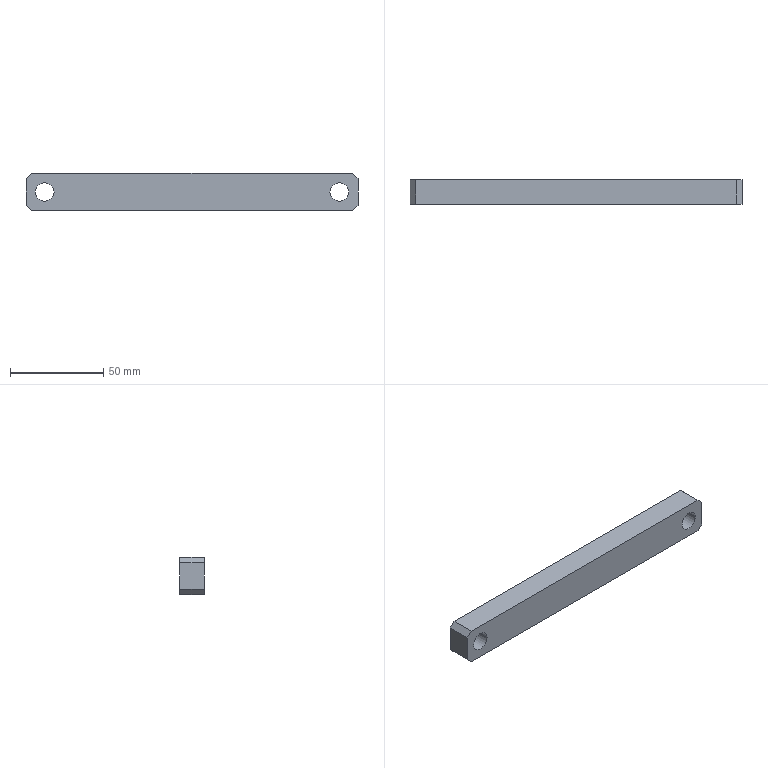Part | SolidWorks | features Chamfer 1, Extrusion 1, ICE 1, LPattern 1 | 1 solid | 14 faces | box 177.8 x 13 x 20 mm | volume 43952 mm3 | plane 10 | cylinder 4 | commonest cylinder face diameters 10 x4
STEP:
#1=CARTESIAN_POINT('',(83.9,-6.5,10.));
#2=VERTEX_POINT('',#1);
#3=CARTESIAN_POINT('',(73.9,-6.5,10.));
#4=VERTEX_POINT('',#3);
#5=CARTESIAN_POINT('',(78.9,-6.5,10.));
#6=DIRECTION('',(0.,1.,0.));
#7=DIRECTION('',(-1.,0.,0.));
#8=AXIS2_PLACEMENT_3D('',#5,#6,#7);
#9=CIRCLE('',#8,5.);
#10=EDGE_CURVE('',#2,#4,#9,.T.);
#11=ORIENTED_EDGE('',*,*,#10,.F.);
#12=CARTESIAN_POINT('',(83.9,6.5,10.));
#13=VERTEX_POINT('',#12);
#14=CARTESIAN_POINT('',(83.9,-6.5,10.));
#15=DIRECTION('',(0.,1.,0.));
#16=VECTOR('',#15,1000.);
#17=LINE('',#14,#16);
#18=EDGE_CURVE('',#2,#13,#17,.T.);
#19=ORIENTED_EDGE('',*,*,#18,.T.);
#20=CARTESIAN_POINT('',(73.9,6.5,10.));
#21=VERTEX_POINT('',#20);
#22=CARTESIAN_POINT('',(78.9,6.5,10.));
#23=DIRECTION('',(0.,1.,0.));
#24=DIRECTION('',(-1.,0.,0.));
#25=AXIS2_PLACEMENT_3D('',#22,#23,#24);
#26=CIRCLE('',#25,5.);
#27=EDGE_CURVE('',#13,#21,#26,.T.);
#28=ORIENTED_EDGE('',*,*,#27,.T.);
#29=CARTESIAN_POINT('',(73.9,-6.5,10.));
#30=DIRECTION('',(0.,1.,0.));
#31=VECTOR('',#30,1000.);
#32=LINE('',#29,#31);
#33=EDGE_CURVE('',#4,#21,#32,.T.);
#34=ORIENTED_EDGE('',*,*,#33,.F.);
#35=EDGE_LOOP('',(#11,#19,#28,#34));
#36=FACE_OUTER_BOUND('',#35,.T.);
#37=CARTESIAN_POINT('',(78.9,-6.5,10.));
#38=DIRECTION('',(0.,1.,0.));
#39=DIRECTION('',(-1.,0.,0.));
#40=AXIS2_PLACEMENT_3D('',#37,#38,#39);
#41=CYLINDRICAL_SURFACE('',#40,5.);
#42=ADVANCED_FACE('',(#36),#41,.F.);
#43=CARTESIAN_POINT('',(-73.9,-6.5,10.));
#44=VERTEX_POINT('',#43);
#45=CARTESIAN_POINT('',(-83.9,-6.5,10.));
#46=VERTEX_POINT('',#45);
#47=CARTESIAN_POINT('',(-78.9,-6.5,10.));
#48=DIRECTION('',(0.,1.,0.));
#49=DIRECTION('',(-1.,0.,0.));
#50=AXIS2_PLACEMENT_3D('',#47,#48,#49);
#51=CIRCLE('',#50,5.);
#52=EDGE_CURVE('',#44,#46,#51,.T.);
#53=ORIENTED_EDGE('',*,*,#52,.F.);
#54=CARTESIAN_POINT('',(-73.9,6.5,10.));
#55=VERTEX_POINT('',#54);
#56=CARTESIAN_POINT('',(-73.9,-6.5,10.));
#57=DIRECTION('',(0.,1.,0.));
#58=VECTOR('',#57,1000.);
#59=LINE('',#56,#58);
#60=EDGE_CURVE('',#44,#55,#59,.T.);
#61=ORIENTED_EDGE('',*,*,#60,.T.);
#62=CARTESIAN_POINT('',(-83.9,6.5,10.));
#63=VERTEX_POINT('',#62);
#64=CARTESIAN_POINT('',(-78.9,6.5,10.));
#65=DIRECTION('',(0.,1.,0.));
#66=DIRECTION('',(-1.,0.,0.));
#67=AXIS2_PLACEMENT_3D('',#64,#65,#66);
#68=CIRCLE('',#67,5.);
#69=EDGE_CURVE('',#55,#63,#68,.T.);
#70=ORIENTED_EDGE('',*,*,#69,.T.);
#71=CARTESIAN_POINT('',(-83.9,-6.5,10.));
#72=DIRECTION('',(0.,1.,0.));
#73=VECTOR('',#72,1000.);
#74=LINE('',#71,#73);
#75=EDGE_CURVE('',#46,#63,#74,.T.);
#76=ORIENTED_EDGE('',*,*,#75,.F.);
#77=EDGE_LOOP('',(#53,#61,#70,#76));
#78=FACE_OUTER_BOUND('',#77,.T.);
#79=CARTESIAN_POINT('',(-78.9,-6.5,10.));
#80=DIRECTION('',(0.,1.,0.));
#81=DIRECTION('',(-1.,0.,0.));
#82=AXIS2_PLACEMENT_3D('',#79,#80,#81);
#83=CYLINDRICAL_SURFACE('',#82,5.);
#84=ADVANCED_FACE('',(#78),#83,.F.);
#85=CARTESIAN_POINT('',(88.9,-6.5,17.));
#86=VERTEX_POINT('',#85);
#87=CARTESIAN_POINT('',(88.9,-6.5,3.));
#88=VERTEX_POINT('',#87);
#89=CARTESIAN_POINT('',(88.9,-6.5,20.));
#90=DIRECTION('',(0.,0.,-1.));
#91=VECTOR('',#90,1000.);
#92=LINE('',#89,#91);
#93=EDGE_CURVE('',#86,#88,#92,.T.);
#94=ORIENTED_EDGE('',*,*,#93,.T.);
#95=CARTESIAN_POINT('',(88.9,6.5,3.));
#96=VERTEX_POINT('',#95);
#97=CARTESIAN_POINT('',(88.9,6.5,3.));
#98=DIRECTION('',(0.,1.,0.));
#99=VECTOR('',#98,1000.);
#100=LINE('',#97,#99);
#101=EDGE_CURVE('',#88,#96,#100,.T.);
#102=ORIENTED_EDGE('',*,*,#101,.T.);
#103=CARTESIAN_POINT('',(88.9,6.5,17.));
#104=VERTEX_POINT('',#103);
#105=CARTESIAN_POINT('',(88.9,6.5,20.));
#106=DIRECTION('',(0.,0.,-1.));
#107=VECTOR('',#106,1000.);
#108=LINE('',#105,#107);
#109=EDGE_CURVE('',#104,#96,#108,.T.);
#110=ORIENTED_EDGE('',*,*,#109,.F.);
#111=CARTESIAN_POINT('',(88.9,-6.5,17.));
#112=DIRECTION('',(0.,-1.,0.));
#113=VECTOR('',#112,1000.);
#114=LINE('',#111,#113);
#115=EDGE_CURVE('',#104,#86,#114,.T.);
#116=ORIENTED_EDGE('',*,*,#115,.T.);
#117=EDGE_LOOP('',(#94,#102,#110,#116));
#118=FACE_OUTER_BOUND('',#117,.T.);
#119=CARTESIAN_POINT('',(88.9,6.5,20.));
#120=DIRECTION('',(-1.,0.,0.));
#121=DIRECTION('',(0.,0.,1.));
#122=AXIS2_PLACEMENT_3D('',#119,#120,#121);
#123=PLANE('',#122);
#124=ADVANCED_FACE('',(#118),#123,.F.);
#125=CARTESIAN_POINT('',(78.9,6.5,10.));
#126=DIRECTION('',(0.,1.,0.));
#127=DIRECTION('',(-1.,0.,0.));
#128=AXIS2_PLACEMENT_3D('',#125,#126,#127);
#129=CIRCLE('',#128,5.);
#130=EDGE_CURVE('',#21,#13,#129,.T.);
#131=ORIENTED_EDGE('',*,*,#130,.F.);
#132=ORIENTED_EDGE('',*,*,#27,.F.);
#133=EDGE_LOOP('',(#131,#132));
#134=FACE_BOUND('',#133,.T.);
#135=CARTESIAN_POINT('',(-78.9,6.5,10.));
#136=DIRECTION('',(0.,1.,0.));
#137=DIRECTION('',(-1.,0.,0.));
#138=AXIS2_PLACEMENT_3D('',#135,#136,#137);
#139=CIRCLE('',#138,5.);
#140=EDGE_CURVE('',#63,#55,#139,.T.);
#141=ORIENTED_EDGE('',*,*,#140,.F.);
#142=ORIENTED_EDGE('',*,*,#69,.F.);
#143=EDGE_LOOP('',(#141,#142));
#144=FACE_BOUND('',#143,.T.);
#145=ORIENTED_EDGE('',*,*,#109,.T.);
#146=CARTESIAN_POINT('',(85.9,6.5,0.));
#147=VERTEX_POINT('',#146);
#148=CARTESIAN_POINT('',(88.9,6.5,3.));
#149=DIRECTION('',(-0.7071,0.,-0.7071));
#150=VECTOR('',#149,1000.);
#151=LINE('',#148,#150);
#152=EDGE_CURVE('',#96,#147,#151,.T.);
#153=ORIENTED_EDGE('',*,*,#152,.T.);
#154=CARTESIAN_POINT('',(-85.9,6.5,0.));
#155=VERTEX_POINT('',#154);
#156=CARTESIAN_POINT('',(-88.9,6.5,0.));
#157=DIRECTION('',(-1.,0.,0.));
#158=VECTOR('',#157,1000.);
#159=LINE('',#156,#158);
#160=EDGE_CURVE('',#147,#155,#159,.T.);
#161=ORIENTED_EDGE('',*,*,#160,.T.);
#162=CARTESIAN_POINT('',(-88.9,6.5,3.));
#163=VERTEX_POINT('',#162);
#164=CARTESIAN_POINT('',(-88.9,6.5,3.));
#165=DIRECTION('',(-0.7071,0.,0.7071));
#166=VECTOR('',#165,1000.);
#167=LINE('',#164,#166);
#168=EDGE_CURVE('',#155,#163,#167,.T.);
#169=ORIENTED_EDGE('',*,*,#168,.T.);
#170=CARTESIAN_POINT('',(-88.9,6.5,17.));
#171=VERTEX_POINT('',#170);
#172=CARTESIAN_POINT('',(-88.9,6.5,20.));
#173=DIRECTION('',(0.,0.,-1.));
#174=VECTOR('',#173,1000.);
#175=LINE('',#172,#174);
#176=EDGE_CURVE('',#171,#163,#175,.T.);
#177=ORIENTED_EDGE('',*,*,#176,.F.);
#178=CARTESIAN_POINT('',(-85.9,6.5,20.));
#179=VERTEX_POINT('',#178);
#180=CARTESIAN_POINT('',(-85.9,6.5,20.));
#181=DIRECTION('',(0.7071,0.,0.7071));
#182=VECTOR('',#181,1000.);
#183=LINE('',#180,#182);
#184=EDGE_CURVE('',#171,#179,#183,.T.);
#185=ORIENTED_EDGE('',*,*,#184,.T.);
#186=CARTESIAN_POINT('',(85.9,6.5,20.));
#187=VERTEX_POINT('',#186);
#188=CARTESIAN_POINT('',(-88.9,6.5,20.));
#189=DIRECTION('',(-1.,0.,0.));
#190=VECTOR('',#189,1000.);
#191=LINE('',#188,#190);
#192=EDGE_CURVE('',#187,#179,#191,.T.);
#193=ORIENTED_EDGE('',*,*,#192,.F.);
#194=CARTESIAN_POINT('',(85.9,6.5,20.));
#195=DIRECTION('',(0.7071,0.,-0.7071));
#196=VECTOR('',#195,1000.);
#197=LINE('',#194,#196);
#198=EDGE_CURVE('',#187,#104,#197,.T.);
#199=ORIENTED_EDGE('',*,*,#198,.T.);
#200=EDGE_LOOP('',(#145,#153,#161,#169,#177,#185,#193,#199));
#201=FACE_OUTER_BOUND('',#200,.T.);
#202=CARTESIAN_POINT('',(-88.9,6.5,20.));
#203=DIRECTION('',(0.,-1.,0.));
#204=DIRECTION('',(0.,0.,-1.));
#205=AXIS2_PLACEMENT_3D('',#202,#203,#204);
#206=PLANE('',#205);
#207=ADVANCED_FACE('',(#134,#144,#201),#206,.F.);
#208=ORIENTED_EDGE('',*,*,#176,.T.);
#209=CARTESIAN_POINT('',(-88.9,-6.5,3.));
#210=VERTEX_POINT('',#209);
#211=CARTESIAN_POINT('',(-88.9,6.5,3.));
#212=DIRECTION('',(0.,-1.,0.));
#213=VECTOR('',#212,1000.);
#214=LINE('',#211,#213);
#215=EDGE_CURVE('',#163,#210,#214,.T.);
#216=ORIENTED_EDGE('',*,*,#215,.T.);
#217=CARTESIAN_POINT('',(-88.9,-6.5,17.));
#218=VERTEX_POINT('',#217);
#219=CARTESIAN_POINT('',(-88.9,-6.5,20.));
#220=DIRECTION('',(0.,0.,-1.));
#221=VECTOR('',#220,1000.);
#222=LINE('',#219,#221);
#223=EDGE_CURVE('',#218,#210,#222,.T.);
#224=ORIENTED_EDGE('',*,*,#223,.F.);
#225=CARTESIAN_POINT('',(-88.9,6.5,17.));
#226=DIRECTION('',(0.,1.,0.));
#227=VECTOR('',#226,1000.);
#228=LINE('',#225,#227);
#229=EDGE_CURVE('',#218,#171,#228,.T.);
#230=ORIENTED_EDGE('',*,*,#229,.T.);
#231=EDGE_LOOP('',(#208,#216,#224,#230));
#232=FACE_OUTER_BOUND('',#231,.T.);
#233=CARTESIAN_POINT('',(-88.9,6.5,20.));
#234=DIRECTION('',(1.,0.,0.));
#235=DIRECTION('',(0.,0.,-1.));
#236=AXIS2_PLACEMENT_3D('',#233,#234,#235);
#237=PLANE('',#236);
#238=ADVANCED_FACE('',(#232),#237,.F.);
#239=CARTESIAN_POINT('',(78.9,-6.5,10.));
#240=DIRECTION('',(0.,1.,0.));
#241=DIRECTION('',(-1.,0.,0.));
#242=AXIS2_PLACEMENT_3D('',#239,#240,#241);
#243=CIRCLE('',#242,5.);
#244=EDGE_CURVE('',#4,#2,#243,.T.);
#245=ORIENTED_EDGE('',*,*,#244,.T.);
#246=ORIENTED_EDGE('',*,*,#10,.T.);
#247=EDGE_LOOP('',(#245,#246));
#248=FACE_BOUND('',#247,.T.);
#249=CARTESIAN_POINT('',(-78.9,-6.5,10.));
#250=DIRECTION('',(0.,1.,0.));
#251=DIRECTION('',(-1.,0.,0.));
#252=AXIS2_PLACEMENT_3D('',#249,#250,#251);
#253=CIRCLE('',#252,5.);
#254=EDGE_CURVE('',#46,#44,#253,.T.);
#255=ORIENTED_EDGE('',*,*,#254,.T.);
#256=ORIENTED_EDGE('',*,*,#52,.T.);
#257=EDGE_LOOP('',(#255,#256));
#258=FACE_BOUND('',#257,.T.);
#259=CARTESIAN_POINT('',(-85.9,-6.5,0.));
#260=VERTEX_POINT('',#259);
#261=CARTESIAN_POINT('',(85.9,-6.5,0.));
#262=VERTEX_POINT('',#261);
#263=CARTESIAN_POINT('',(-88.9,-6.5,0.));
#264=DIRECTION('',(1.,0.,0.));
#265=VECTOR('',#264,1000.);
#266=LINE('',#263,#265);
#267=EDGE_CURVE('',#260,#262,#266,.T.);
#268=ORIENTED_EDGE('',*,*,#267,.T.);
#269=CARTESIAN_POINT('',(88.9,-6.5,3.));
#270=DIRECTION('',(0.7071,0.,0.7071));
#271=VECTOR('',#270,1000.);
#272=LINE('',#269,#271);
#273=EDGE_CURVE('',#262,#88,#272,.T.);
#274=ORIENTED_EDGE('',*,*,#273,.T.);
#275=ORIENTED_EDGE('',*,*,#93,.F.);
#276=CARTESIAN_POINT('',(85.9,-6.5,20.));
#277=VERTEX_POINT('',#276);
#278=CARTESIAN_POINT('',(85.9,-6.5,20.));
#279=DIRECTION('',(-0.7071,0.,0.7071));
#280=VECTOR('',#279,1000.);
#281=LINE('',#278,#280);
#282=EDGE_CURVE('',#86,#277,#281,.T.);
#283=ORIENTED_EDGE('',*,*,#282,.T.);
#284=CARTESIAN_POINT('',(-85.9,-6.5,20.));
#285=VERTEX_POINT('',#284);
#286=CARTESIAN_POINT('',(-88.9,-6.5,20.));
#287=DIRECTION('',(1.,0.,0.));
#288=VECTOR('',#287,1000.);
#289=LINE('',#286,#288);
#290=EDGE_CURVE('',#285,#277,#289,.T.);
#291=ORIENTED_EDGE('',*,*,#290,.F.);
#292=CARTESIAN_POINT('',(-85.9,-6.5,20.));
#293=DIRECTION('',(-0.7071,0.,-0.7071));
#294=VECTOR('',#293,1000.);
#295=LINE('',#292,#294);
#296=EDGE_CURVE('',#285,#218,#295,.T.);
#297=ORIENTED_EDGE('',*,*,#296,.T.);
#298=ORIENTED_EDGE('',*,*,#223,.T.);
#299=CARTESIAN_POINT('',(-88.9,-6.5,3.));
#300=DIRECTION('',(0.7071,0.,-0.7071));
#301=VECTOR('',#300,1000.);
#302=LINE('',#299,#301);
#303=EDGE_CURVE('',#210,#260,#302,.T.);
#304=ORIENTED_EDGE('',*,*,#303,.T.);
#305=EDGE_LOOP('',(#268,#274,#275,#283,#291,#297,#298,#304));
#306=FACE_OUTER_BOUND('',#305,.T.);
#307=CARTESIAN_POINT('',(-88.9,-6.5,20.));
#308=DIRECTION('',(0.,1.,0.));
#309=DIRECTION('',(0.,0.,1.));
#310=AXIS2_PLACEMENT_3D('',#307,#308,#309);
#311=PLANE('',#310);
#312=ADVANCED_FACE('',(#248,#258,#306),#311,.F.);
#313=ORIENTED_EDGE('',*,*,#192,.T.);
#314=CARTESIAN_POINT('',(-85.9,-6.5,20.));
#315=DIRECTION('',(0.,-1.,0.));
#316=VECTOR('',#315,1000.);
#317=LINE('',#314,#316);
#318=EDGE_CURVE('',#179,#285,#317,.T.);
#319=ORIENTED_EDGE('',*,*,#318,.T.);
#320=ORIENTED_EDGE('',*,*,#290,.T.);
#321=CARTESIAN_POINT('',(85.9,6.5,20.));
#322=DIRECTION('',(0.,1.,0.));
#323=VECTOR('',#322,1000.);
#324=LINE('',#321,#323);
#325=EDGE_CURVE('',#277,#187,#324,.T.);
#326=ORIENTED_EDGE('',*,*,#325,.T.);
#327=EDGE_LOOP('',(#313,#319,#320,#326));
#328=FACE_OUTER_BOUND('',#327,.T.);
#329=CARTESIAN_POINT('',(0.,0.,20.));
#330=DIRECTION('',(0.,0.,1.));
#331=DIRECTION('',(1.,0.,0.));
#332=AXIS2_PLACEMENT_3D('',#329,#330,#331);
#333=PLANE('',#332);
#334=ADVANCED_FACE('',(#328),#333,.T.);
#335=ORIENTED_EDGE('',*,*,#160,.F.);
#336=CARTESIAN_POINT('',(85.9,0.,0.));
#337=DIRECTION('',(0.,-1.,0.));
#338=VECTOR('',#337,1000.);
#339=LINE('',#336,#338);
#340=EDGE_CURVE('',#147,#262,#339,.T.);
#341=ORIENTED_EDGE('',*,*,#340,.T.);
#342=ORIENTED_EDGE('',*,*,#267,.F.);
#343=CARTESIAN_POINT('',(-85.9,0.,0.));
#344=DIRECTION('',(0.,1.,0.));
#345=VECTOR('',#344,1000.);
#346=LINE('',#343,#345);
#347=EDGE_CURVE('',#260,#155,#346,.T.);
#348=ORIENTED_EDGE('',*,*,#347,.T.);
#349=EDGE_LOOP('',(#335,#341,#342,#348));
#350=FACE_OUTER_BOUND('',#349,.T.);
#351=CARTESIAN_POINT('',(0.,0.,0.));
#352=DIRECTION('',(0.,0.,1.));
#353=DIRECTION('',(1.,0.,0.));
#354=AXIS2_PLACEMENT_3D('',#351,#352,#353);
#355=PLANE('',#354);
#356=ADVANCED_FACE('',(#350),#355,.F.);
#357=ORIENTED_EDGE('',*,*,#273,.F.);
#358=ORIENTED_EDGE('',*,*,#340,.F.);
#359=ORIENTED_EDGE('',*,*,#152,.F.);
#360=ORIENTED_EDGE('',*,*,#101,.F.);
#361=EDGE_LOOP('',(#357,#358,#359,#360));
#362=FACE_OUTER_BOUND('',#361,.T.);
#363=CARTESIAN_POINT('',(88.9,6.5,3.));
#364=DIRECTION('',(-0.7071,0.,0.7071));
#365=DIRECTION('',(0.,1.,0.));
#366=AXIS2_PLACEMENT_3D('',#363,#364,#365);
#367=PLANE('',#366);
#368=ADVANCED_FACE('',(#362),#367,.F.);
#369=ORIENTED_EDGE('',*,*,#168,.F.);
#370=ORIENTED_EDGE('',*,*,#347,.F.);
#371=ORIENTED_EDGE('',*,*,#303,.F.);
#372=ORIENTED_EDGE('',*,*,#215,.F.);
#373=EDGE_LOOP('',(#369,#370,#371,#372));
#374=FACE_OUTER_BOUND('',#373,.T.);
#375=CARTESIAN_POINT('',(-88.9,6.5,3.));
#376=DIRECTION('',(0.7071,0.,0.7071));
#377=DIRECTION('',(0.,-1.,0.));
#378=AXIS2_PLACEMENT_3D('',#375,#376,#377);
#379=PLANE('',#378);
#380=ADVANCED_FACE('',(#374),#379,.F.);
#381=ORIENTED_EDGE('',*,*,#184,.F.);
#382=ORIENTED_EDGE('',*,*,#229,.F.);
#383=ORIENTED_EDGE('',*,*,#296,.F.);
#384=ORIENTED_EDGE('',*,*,#318,.F.);
#385=EDGE_LOOP('',(#381,#382,#383,#384));
#386=FACE_OUTER_BOUND('',#385,.T.);
#387=CARTESIAN_POINT('',(-85.9,0.,20.));
#388=DIRECTION('',(-0.7071,0.,0.7071));
#389=DIRECTION('',(0.,1.,0.));
#390=AXIS2_PLACEMENT_3D('',#387,#388,#389);
#391=PLANE('',#390);
#392=ADVANCED_FACE('',(#386),#391,.T.);
#393=ORIENTED_EDGE('',*,*,#282,.F.);
#394=ORIENTED_EDGE('',*,*,#115,.F.);
#395=ORIENTED_EDGE('',*,*,#198,.F.);
#396=ORIENTED_EDGE('',*,*,#325,.F.);
#397=EDGE_LOOP('',(#393,#394,#395,#396));
#398=FACE_OUTER_BOUND('',#397,.T.);
#399=CARTESIAN_POINT('',(85.9,0.,20.));
#400=DIRECTION('',(0.7071,0.,0.7071));
#401=DIRECTION('',(0.,-1.,0.));
#402=AXIS2_PLACEMENT_3D('',#399,#400,#401);
#403=PLANE('',#402);
#404=ADVANCED_FACE('',(#398),#403,.T.);
#405=ORIENTED_EDGE('',*,*,#60,.F.);
#406=ORIENTED_EDGE('',*,*,#254,.F.);
#407=ORIENTED_EDGE('',*,*,#75,.T.);
#408=ORIENTED_EDGE('',*,*,#140,.T.);
#409=EDGE_LOOP('',(#405,#406,#407,#408));
#410=FACE_OUTER_BOUND('',#409,.T.);
#411=CARTESIAN_POINT('',(-78.9,-6.5,10.));
#412=DIRECTION('',(0.,1.,0.));
#413=DIRECTION('',(-1.,0.,0.));
#414=AXIS2_PLACEMENT_3D('',#411,#412,#413);
#415=CYLINDRICAL_SURFACE('',#414,5.);
#416=ADVANCED_FACE('',(#410),#415,.F.);
#417=ORIENTED_EDGE('',*,*,#18,.F.);
#418=ORIENTED_EDGE('',*,*,#244,.F.);
#419=ORIENTED_EDGE('',*,*,#33,.T.);
#420=ORIENTED_EDGE('',*,*,#130,.T.);
#421=EDGE_LOOP('',(#417,#418,#419,#420));
#422=FACE_OUTER_BOUND('',#421,.T.);
#423=CARTESIAN_POINT('',(78.9,-6.5,10.));
#424=DIRECTION('',(0.,1.,0.));
#425=DIRECTION('',(-1.,0.,0.));
#426=AXIS2_PLACEMENT_3D('',#423,#424,#425);
#427=CYLINDRICAL_SURFACE('',#426,5.);
#428=ADVANCED_FACE('',(#422),#427,.F.);
#429=CLOSED_SHELL('',(#42,#84,#124,#207,#238,#312,#334,#356,#368,#380,#392,#404,#416,#428));
#430=MANIFOLD_SOLID_BREP('',#429);
#431=CARTESIAN_POINT('',(0.,0.,0.));
#432=DIRECTION('',(0.,0.,1.));
#433=DIRECTION('',(1.,0.,0.));
#434=AXIS2_PLACEMENT_3D('',#431,#432,#433);
#435=(LENGTH_UNIT()NAMED_UNIT(*)SI_UNIT(.MILLI.,.METRE.));
#436=UNCERTAINTY_MEASURE_WITH_UNIT(LENGTH_MEASURE(0.00001),#435,'','');
#437=(NAMED_UNIT(*)PLANE_ANGLE_UNIT()SI_UNIT($,.RADIAN.));
#438=(NAMED_UNIT(*)SI_UNIT($,.STERADIAN.)SOLID_ANGLE_UNIT());
#439=(GEOMETRIC_REPRESENTATION_CONTEXT(3)GLOBAL_UNCERTAINTY_ASSIGNED_CONTEXT((#436))GLOBAL_UNIT_ASSIGNED_CONTEXT((#435,#437,#438))REPRESENTATION_CONTEXT('',''));
#440=ADVANCED_BREP_SHAPE_REPRESENTATION('',(#430,#434),#439);